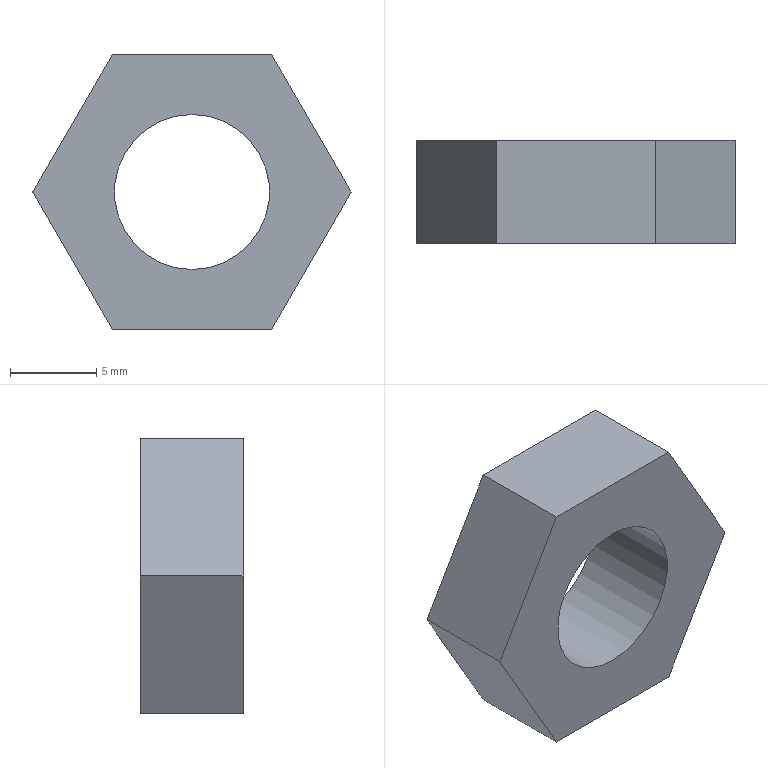Part | NX | 1 solid | 9 faces | box 18.475 x 6 x 16 mm | volume 948.512 mm3 | plane 8 | cylinder 1 | commonest cylinder face diameters 9 x1
STEP:
#1=CARTESIAN_POINT('',(4.619,0.,8.));
#2=VERTEX_POINT('',#1);
#3=CARTESIAN_POINT('',(9.238,0.,0.));
#4=VERTEX_POINT('',#3);
#5=CARTESIAN_POINT('',(4.619,0.,8.));
#6=DIRECTION('',(0.5,0.,-0.866));
#7=VECTOR('',#6,1000.);
#8=LINE('',#5,#7);
#9=EDGE_CURVE('',#2,#4,#8,.T.);
#10=ORIENTED_EDGE('',*,*,#9,.T.);
#11=CARTESIAN_POINT('',(9.238,6.,0.));
#12=VERTEX_POINT('',#11);
#13=CARTESIAN_POINT('',(9.238,6.,0.));
#14=DIRECTION('',(0.,-1.,0.));
#15=VECTOR('',#14,1000.);
#16=LINE('',#13,#15);
#17=EDGE_CURVE('',#12,#4,#16,.T.);
#18=ORIENTED_EDGE('',*,*,#17,.F.);
#19=CARTESIAN_POINT('',(4.619,6.,8.));
#20=VERTEX_POINT('',#19);
#21=CARTESIAN_POINT('',(4.619,6.,8.));
#22=DIRECTION('',(0.5,0.,-0.866));
#23=VECTOR('',#22,1000.);
#24=LINE('',#21,#23);
#25=EDGE_CURVE('',#20,#12,#24,.T.);
#26=ORIENTED_EDGE('',*,*,#25,.F.);
#27=CARTESIAN_POINT('',(4.619,6.,8.));
#28=DIRECTION('',(0.,-1.,0.));
#29=VECTOR('',#28,1000.);
#30=LINE('',#27,#29);
#31=EDGE_CURVE('',#20,#2,#30,.T.);
#32=ORIENTED_EDGE('',*,*,#31,.T.);
#33=EDGE_LOOP('',(#10,#18,#26,#32));
#34=FACE_BOUND('',#33,.T.);
#35=CARTESIAN_POINT('',(4.619,6.,8.));
#36=DIRECTION('',(-0.866,0.,-0.5));
#37=DIRECTION('',(-0.5,0.,0.866));
#38=AXIS2_PLACEMENT_3D('',#35,#36,#37);
#39=PLANE('',#38);
#40=ADVANCED_FACE('',(#34),#39,.F.);
#41=CARTESIAN_POINT('',(4.619,0.,-8.));
#42=VERTEX_POINT('',#41);
#43=CARTESIAN_POINT('',(9.238,0.,0.));
#44=DIRECTION('',(-0.5,0.,-0.866));
#45=VECTOR('',#44,1000.);
#46=LINE('',#43,#45);
#47=EDGE_CURVE('',#4,#42,#46,.T.);
#48=ORIENTED_EDGE('',*,*,#47,.T.);
#49=CARTESIAN_POINT('',(4.619,6.,-8.));
#50=VERTEX_POINT('',#49);
#51=CARTESIAN_POINT('',(4.619,6.,-8.));
#52=DIRECTION('',(0.,-1.,0.));
#53=VECTOR('',#52,1000.);
#54=LINE('',#51,#53);
#55=EDGE_CURVE('',#50,#42,#54,.T.);
#56=ORIENTED_EDGE('',*,*,#55,.F.);
#57=CARTESIAN_POINT('',(9.238,6.,0.));
#58=DIRECTION('',(-0.5,0.,-0.866));
#59=VECTOR('',#58,1000.);
#60=LINE('',#57,#59);
#61=EDGE_CURVE('',#12,#50,#60,.T.);
#62=ORIENTED_EDGE('',*,*,#61,.F.);
#63=ORIENTED_EDGE('',*,*,#17,.T.);
#64=EDGE_LOOP('',(#48,#56,#62,#63));
#65=FACE_BOUND('',#64,.T.);
#66=CARTESIAN_POINT('',(9.238,6.,0.));
#67=DIRECTION('',(-0.866,0.,0.5));
#68=DIRECTION('',(0.5,0.,0.866));
#69=AXIS2_PLACEMENT_3D('',#66,#67,#68);
#70=PLANE('',#69);
#71=ADVANCED_FACE('',(#65),#70,.F.);
#72=CARTESIAN_POINT('',(-4.619,0.,-8.));
#73=VERTEX_POINT('',#72);
#74=CARTESIAN_POINT('',(4.619,0.,-8.));
#75=DIRECTION('',(-1.,0.,0.));
#76=VECTOR('',#75,1000.);
#77=LINE('',#74,#76);
#78=EDGE_CURVE('',#42,#73,#77,.T.);
#79=ORIENTED_EDGE('',*,*,#78,.T.);
#80=CARTESIAN_POINT('',(-4.619,6.,-8.));
#81=VERTEX_POINT('',#80);
#82=CARTESIAN_POINT('',(-4.619,6.,-8.));
#83=DIRECTION('',(0.,-1.,0.));
#84=VECTOR('',#83,1000.);
#85=LINE('',#82,#84);
#86=EDGE_CURVE('',#81,#73,#85,.T.);
#87=ORIENTED_EDGE('',*,*,#86,.F.);
#88=CARTESIAN_POINT('',(4.619,6.,-8.));
#89=DIRECTION('',(-1.,0.,0.));
#90=VECTOR('',#89,1000.);
#91=LINE('',#88,#90);
#92=EDGE_CURVE('',#50,#81,#91,.T.);
#93=ORIENTED_EDGE('',*,*,#92,.F.);
#94=ORIENTED_EDGE('',*,*,#55,.T.);
#95=EDGE_LOOP('',(#79,#87,#93,#94));
#96=FACE_BOUND('',#95,.T.);
#97=CARTESIAN_POINT('',(4.619,6.,-8.));
#98=DIRECTION('',(0.,0.,1.));
#99=DIRECTION('',(1.,0.,0.));
#100=AXIS2_PLACEMENT_3D('',#97,#98,#99);
#101=PLANE('',#100);
#102=ADVANCED_FACE('',(#96),#101,.F.);
#103=CARTESIAN_POINT('',(-9.238,0.,0.));
#104=VERTEX_POINT('',#103);
#105=CARTESIAN_POINT('',(-4.619,0.,-8.));
#106=DIRECTION('',(-0.5,0.,0.866));
#107=VECTOR('',#106,1000.);
#108=LINE('',#105,#107);
#109=EDGE_CURVE('',#73,#104,#108,.T.);
#110=ORIENTED_EDGE('',*,*,#109,.T.);
#111=CARTESIAN_POINT('',(-9.238,6.,0.));
#112=VERTEX_POINT('',#111);
#113=CARTESIAN_POINT('',(-9.238,6.,0.));
#114=DIRECTION('',(0.,-1.,0.));
#115=VECTOR('',#114,1000.);
#116=LINE('',#113,#115);
#117=EDGE_CURVE('',#112,#104,#116,.T.);
#118=ORIENTED_EDGE('',*,*,#117,.F.);
#119=CARTESIAN_POINT('',(-4.619,6.,-8.));
#120=DIRECTION('',(-0.5,0.,0.866));
#121=VECTOR('',#120,1000.);
#122=LINE('',#119,#121);
#123=EDGE_CURVE('',#81,#112,#122,.T.);
#124=ORIENTED_EDGE('',*,*,#123,.F.);
#125=ORIENTED_EDGE('',*,*,#86,.T.);
#126=EDGE_LOOP('',(#110,#118,#124,#125));
#127=FACE_BOUND('',#126,.T.);
#128=CARTESIAN_POINT('',(-4.619,6.,-8.));
#129=DIRECTION('',(0.866,0.,0.5));
#130=DIRECTION('',(0.5,0.,-0.866));
#131=AXIS2_PLACEMENT_3D('',#128,#129,#130);
#132=PLANE('',#131);
#133=ADVANCED_FACE('',(#127),#132,.F.);
#134=CARTESIAN_POINT('',(-4.619,0.,8.));
#135=VERTEX_POINT('',#134);
#136=CARTESIAN_POINT('',(-9.238,0.,0.));
#137=DIRECTION('',(0.5,0.,0.866));
#138=VECTOR('',#137,1000.);
#139=LINE('',#136,#138);
#140=EDGE_CURVE('',#104,#135,#139,.T.);
#141=ORIENTED_EDGE('',*,*,#140,.T.);
#142=CARTESIAN_POINT('',(-4.619,6.,8.));
#143=VERTEX_POINT('',#142);
#144=CARTESIAN_POINT('',(-4.619,6.,8.));
#145=DIRECTION('',(0.,-1.,0.));
#146=VECTOR('',#145,1000.);
#147=LINE('',#144,#146);
#148=EDGE_CURVE('',#143,#135,#147,.T.);
#149=ORIENTED_EDGE('',*,*,#148,.F.);
#150=CARTESIAN_POINT('',(-9.238,6.,0.));
#151=DIRECTION('',(0.5,0.,0.866));
#152=VECTOR('',#151,1000.);
#153=LINE('',#150,#152);
#154=EDGE_CURVE('',#112,#143,#153,.T.);
#155=ORIENTED_EDGE('',*,*,#154,.F.);
#156=ORIENTED_EDGE('',*,*,#117,.T.);
#157=EDGE_LOOP('',(#141,#149,#155,#156));
#158=FACE_BOUND('',#157,.T.);
#159=CARTESIAN_POINT('',(-9.238,6.,0.));
#160=DIRECTION('',(0.866,0.,-0.5));
#161=DIRECTION('',(-0.5,0.,-0.866));
#162=AXIS2_PLACEMENT_3D('',#159,#160,#161);
#163=PLANE('',#162);
#164=ADVANCED_FACE('',(#158),#163,.F.);
#165=CARTESIAN_POINT('',(-4.619,0.,8.));
#166=DIRECTION('',(1.,0.,0.));
#167=VECTOR('',#166,1000.);
#168=LINE('',#165,#167);
#169=EDGE_CURVE('',#135,#2,#168,.T.);
#170=ORIENTED_EDGE('',*,*,#169,.T.);
#171=ORIENTED_EDGE('',*,*,#31,.F.);
#172=CARTESIAN_POINT('',(-4.619,6.,8.));
#173=DIRECTION('',(1.,0.,0.));
#174=VECTOR('',#173,1000.);
#175=LINE('',#172,#174);
#176=EDGE_CURVE('',#143,#20,#175,.T.);
#177=ORIENTED_EDGE('',*,*,#176,.F.);
#178=ORIENTED_EDGE('',*,*,#148,.T.);
#179=EDGE_LOOP('',(#170,#171,#177,#178));
#180=FACE_BOUND('',#179,.T.);
#181=CARTESIAN_POINT('',(-4.619,6.,8.));
#182=DIRECTION('',(0.,0.,-1.));
#183=DIRECTION('',(-1.,0.,0.));
#184=AXIS2_PLACEMENT_3D('',#181,#182,#183);
#185=PLANE('',#184);
#186=ADVANCED_FACE('',(#180),#185,.F.);
#187=CARTESIAN_POINT('',(0.,6.,4.5));
#188=VERTEX_POINT('',#187);
#189=CARTESIAN_POINT('',(0.,6.,0.));
#190=DIRECTION('',(0.,1.,0.));
#191=DIRECTION('',(0.,0.,1.));
#192=AXIS2_PLACEMENT_3D('',#189,#190,#191);
#193=CIRCLE('',#192,4.5);
#194=EDGE_CURVE('',#188,#188,#193,.T.);
#195=ORIENTED_EDGE('',*,*,#194,.F.);
#196=EDGE_LOOP('',(#195));
#197=FACE_BOUND('',#196,.T.);
#198=ORIENTED_EDGE('',*,*,#25,.T.);
#199=ORIENTED_EDGE('',*,*,#61,.T.);
#200=ORIENTED_EDGE('',*,*,#92,.T.);
#201=ORIENTED_EDGE('',*,*,#123,.T.);
#202=ORIENTED_EDGE('',*,*,#154,.T.);
#203=ORIENTED_EDGE('',*,*,#176,.T.);
#204=EDGE_LOOP('',(#198,#199,#200,#201,#202,#203));
#205=FACE_BOUND('',#204,.T.);
#206=CARTESIAN_POINT('',(0.,6.,0.));
#207=DIRECTION('',(0.,1.,0.));
#208=DIRECTION('',(0.,0.,1.));
#209=AXIS2_PLACEMENT_3D('',#206,#207,#208);
#210=PLANE('',#209);
#211=ADVANCED_FACE('',(#197,#205),#210,.T.);
#212=CARTESIAN_POINT('',(0.,0.,4.5));
#213=VERTEX_POINT('',#212);
#214=CARTESIAN_POINT('',(0.,0.,0.));
#215=DIRECTION('',(0.,1.,0.));
#216=DIRECTION('',(0.,0.,1.));
#217=AXIS2_PLACEMENT_3D('',#214,#215,#216);
#218=CIRCLE('',#217,4.5);
#219=EDGE_CURVE('',#213,#213,#218,.T.);
#220=ORIENTED_EDGE('',*,*,#219,.T.);
#221=EDGE_LOOP('',(#220));
#222=FACE_BOUND('',#221,.T.);
#223=ORIENTED_EDGE('',*,*,#9,.F.);
#224=ORIENTED_EDGE('',*,*,#169,.F.);
#225=ORIENTED_EDGE('',*,*,#140,.F.);
#226=ORIENTED_EDGE('',*,*,#109,.F.);
#227=ORIENTED_EDGE('',*,*,#78,.F.);
#228=ORIENTED_EDGE('',*,*,#47,.F.);
#229=EDGE_LOOP('',(#223,#224,#225,#226,#227,#228));
#230=FACE_BOUND('',#229,.T.);
#231=CARTESIAN_POINT('',(0.,0.,0.));
#232=DIRECTION('',(0.,1.,0.));
#233=DIRECTION('',(0.,0.,1.));
#234=AXIS2_PLACEMENT_3D('',#231,#232,#233);
#235=PLANE('',#234);
#236=ADVANCED_FACE('',(#222,#230),#235,.F.);
#237=ORIENTED_EDGE('',*,*,#219,.F.);
#238=EDGE_LOOP('',(#237));
#239=FACE_BOUND('',#238,.T.);
#240=ORIENTED_EDGE('',*,*,#194,.T.);
#241=EDGE_LOOP('',(#240));
#242=FACE_BOUND('',#241,.T.);
#243=CARTESIAN_POINT('',(0.,6.,0.));
#244=DIRECTION('',(0.,1.,0.));
#245=DIRECTION('',(0.,0.,1.));
#246=AXIS2_PLACEMENT_3D('',#243,#244,#245);
#247=CYLINDRICAL_SURFACE('',#246,4.5);
#248=ADVANCED_FACE('',(#239,#242),#247,.F.);
#249=CLOSED_SHELL('',(#40,#71,#102,#133,#164,#186,#211,#236,#248));
#250=MANIFOLD_SOLID_BREP('',#249);
#251=(LENGTH_UNIT()NAMED_UNIT(*)SI_UNIT(.MILLI.,.METRE.));
#252=UNCERTAINTY_MEASURE_WITH_UNIT(LENGTH_MEASURE(0.00001),#251,'','');
#253=(NAMED_UNIT(*)PLANE_ANGLE_UNIT()SI_UNIT($,.RADIAN.));
#254=(NAMED_UNIT(*)SI_UNIT($,.STERADIAN.)SOLID_ANGLE_UNIT());
#255=(GEOMETRIC_REPRESENTATION_CONTEXT(3)GLOBAL_UNCERTAINTY_ASSIGNED_CONTEXT((#252))GLOBAL_UNIT_ASSIGNED_CONTEXT((#251,#253,#254))REPRESENTATION_CONTEXT('',''));
#256=ADVANCED_BREP_SHAPE_REPRESENTATION('',(#250),#255);